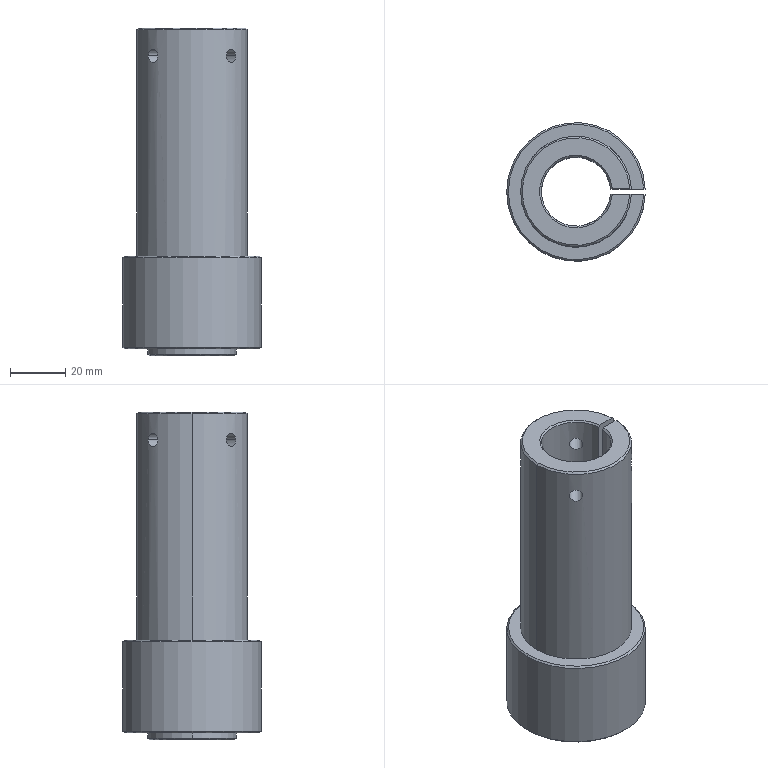Part | SolidWorks | features ICE 6, MoveFace 4, HoleWzd 2, Chamfer 1, CirPattern 1, DelFace 1, Extrusion 1, MirrorPattern 1 | 1 solid | 46 faces | box 49.98 x 50 x 118.2 mm | volume 109781 mm3 | cylinder 23 | cone 17 | plane 6 | commonest cylinder face diameters 3.3 x8 4.8 x8 25 x2 32 x2 40 x2 50 x1